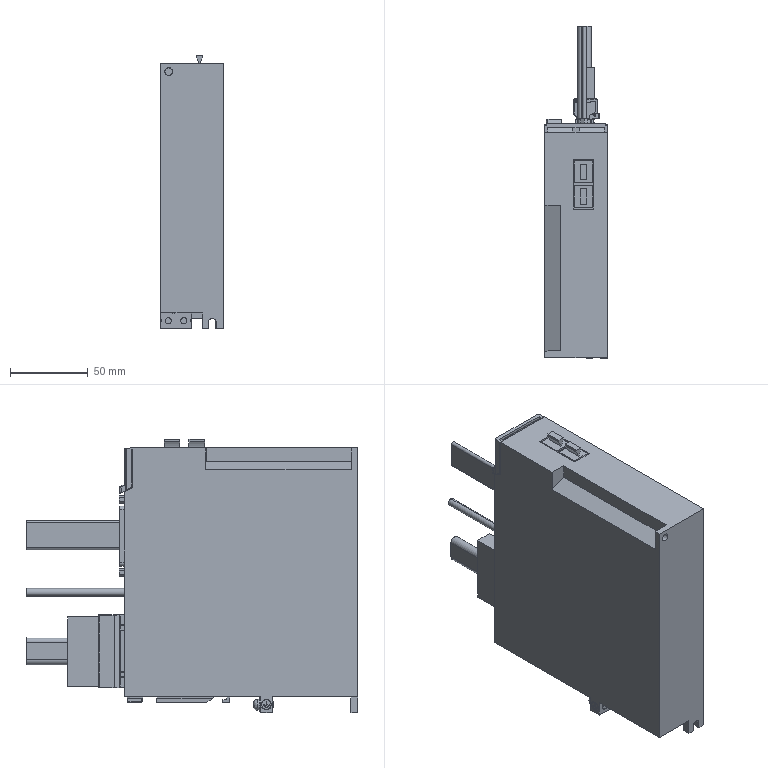Part | STEP file | servo drive SV660PS1R6I | 6 solids | 1414 faces | box 40 x 213 x 175.4 mm | volume 974697 mm3 | plane 939 | cylinder 395 | sphere 26 | spline 26 | cone 17 | torus 11 | commonest cylinder face diameters 1 x130 0.6 x104 0.4 x35 4 x14 3.6 x13 0.2 x12